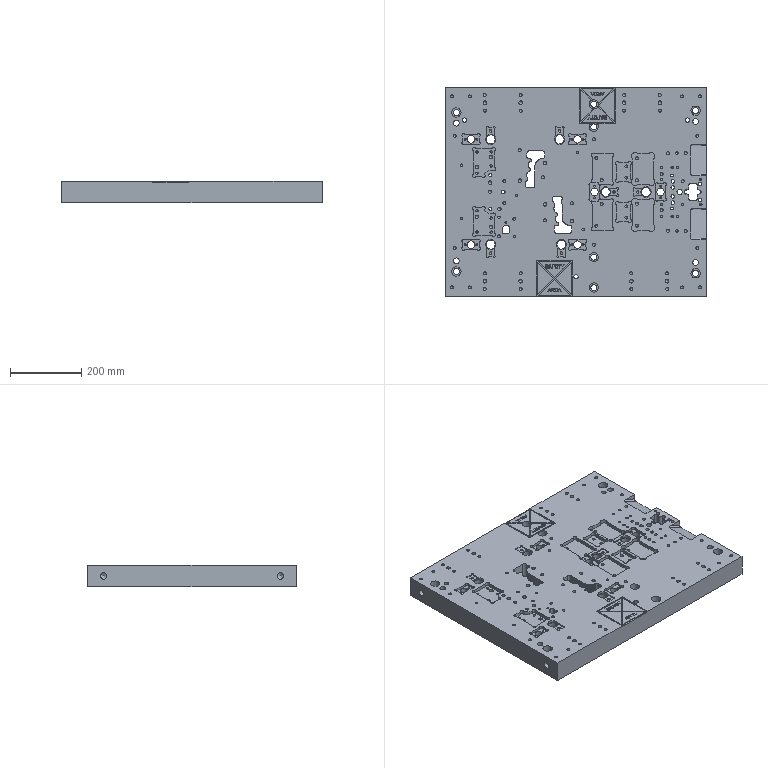Part | STEP file | 1 solid | 1220 faces | box 730 x 585 x 60 mm | volume 23773121 mm3 | plane 719 | cylinder 319 | cone 143 | spline 39 | commonest cylinder face diameters 10 x79 8.5 x49 6.8 x33 6 x22 14 x19 8 x14